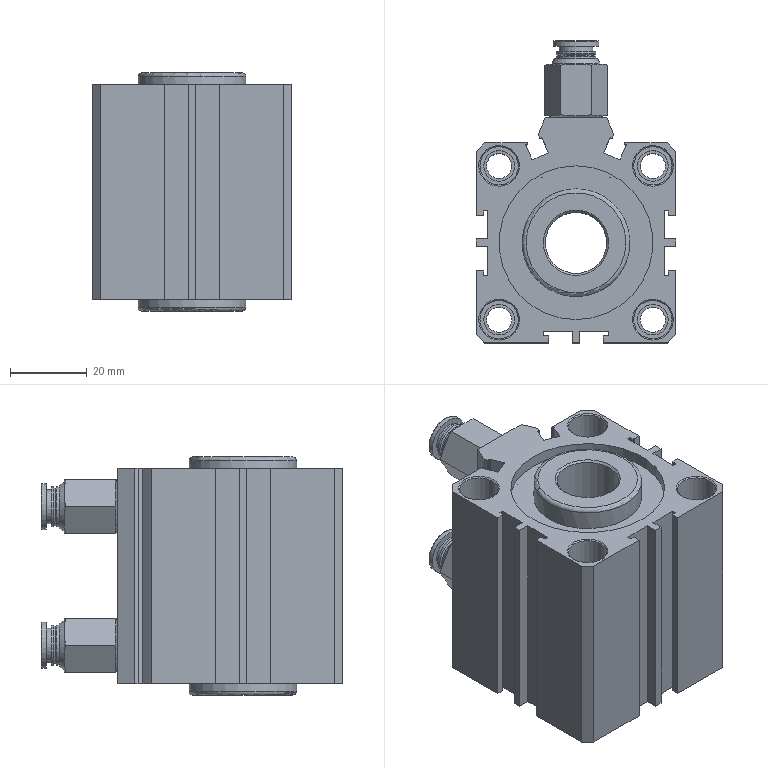Part | STEP file | 冲床-300配套压波_id658_x_t | 1 solid | 211 faces | box 52 x 78.5 x 62 mm | volume 126895 mm3 | plane 114 | cylinder 69 | cone 20 | torus 8 | commonest cylinder face diameters 0.4 x30 8 x10 10 x8 6.5 x4 10.4 x4 8.23 x2